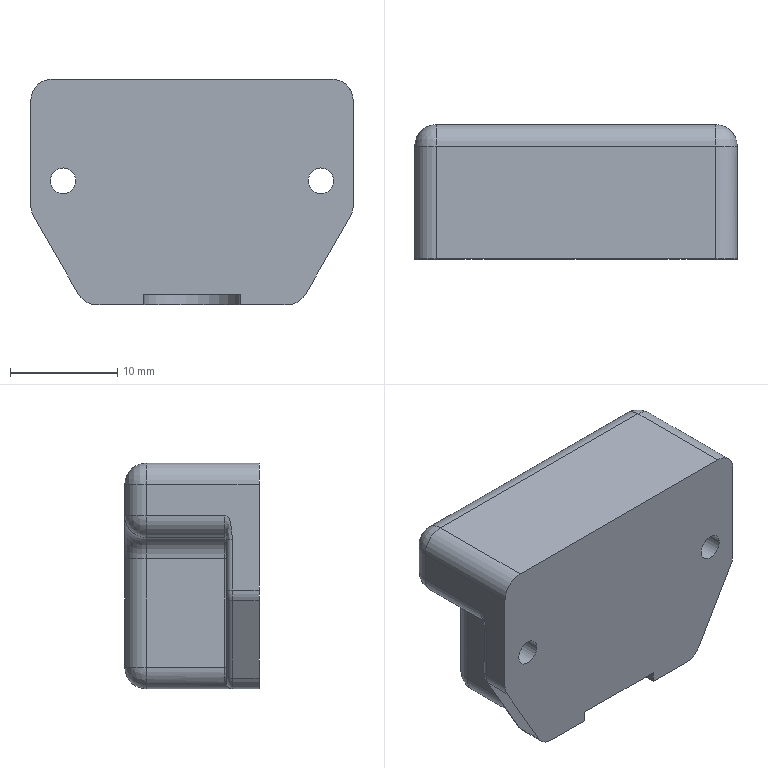Part | STEP file | 1 solid | 72 faces | box 30 x 12.5 x 21 mm | volume 6057 mm3 | cylinder 33 | plane 17 | torus 10 | spline 6 | sphere 6 | commonest cylinder face diameters 4 x20 1 x6 0.4 x4 2.373 x2 9 x1